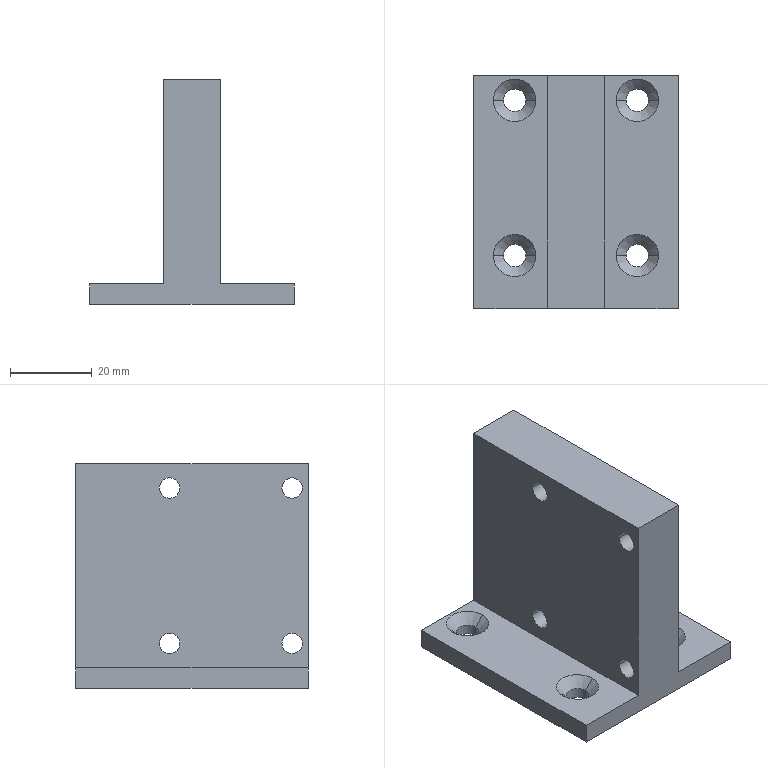Part | 1 solid | 34 faces | box 50 x 57 x 55 mm | volume 52306 mm3 | cylinder 16 | plane 10 | cone 8 | commonest cylinder face diameters 5 x8 5.5 x8
STEP:
#1=CARTESIAN_POINT('',(7.25,41.,2.55));
#2=VERTEX_POINT('',#1);
#3=CARTESIAN_POINT('',(12.75,41.,2.55));
#4=VERTEX_POINT('',#3);
#5=CARTESIAN_POINT('',(10.,41.,2.55));
#6=DIRECTION('',(0.,0.,1.));
#7=DIRECTION('',(1.,0.,0.));
#8=AXIS2_PLACEMENT_3D('',#5,#6,#7);
#9=CIRCLE('',#8,2.75);
#10=EDGE_CURVE('',#2,#4,#9,.T.);
#11=ORIENTED_EDGE('',*,*,#10,.F.);
#12=CARTESIAN_POINT('',(4.8,41.,5.));
#13=VERTEX_POINT('',#12);
#14=CARTESIAN_POINT('',(4.8,41.,5.));
#15=DIRECTION('',(-0.7071,0.,0.7071));
#16=VECTOR('',#15,1000.);
#17=LINE('',#14,#16);
#18=EDGE_CURVE('',#2,#13,#17,.T.);
#19=ORIENTED_EDGE('',*,*,#18,.T.);
#20=CARTESIAN_POINT('',(15.2,41.,5.));
#21=VERTEX_POINT('',#20);
#22=CARTESIAN_POINT('',(10.,41.,5.));
#23=DIRECTION('',(0.,0.,1.));
#24=DIRECTION('',(1.,0.,0.));
#25=AXIS2_PLACEMENT_3D('',#22,#23,#24);
#26=CIRCLE('',#25,5.2);
#27=EDGE_CURVE('',#13,#21,#26,.T.);
#28=ORIENTED_EDGE('',*,*,#27,.T.);
#29=CARTESIAN_POINT('',(15.2,41.,5.));
#30=DIRECTION('',(0.7071,0.,0.7071));
#31=VECTOR('',#30,1000.);
#32=LINE('',#29,#31);
#33=EDGE_CURVE('',#4,#21,#32,.T.);
#34=ORIENTED_EDGE('',*,*,#33,.F.);
#35=EDGE_LOOP('',(#11,#19,#28,#34));
#36=FACE_OUTER_BOUND('',#35,.T.);
#37=CARTESIAN_POINT('',(10.,41.,5.));
#38=DIRECTION('',(0.,0.,1.));
#39=DIRECTION('',(1.,0.,0.));
#40=AXIS2_PLACEMENT_3D('',#37,#38,#39);
#41=CONICAL_SURFACE('',#40,5.2,0.7854);
#42=ADVANCED_FACE('',(#36),#41,.F.);
#43=CARTESIAN_POINT('',(12.75,41.,0.));
#44=VERTEX_POINT('',#43);
#45=CARTESIAN_POINT('',(7.25,41.,0.));
#46=VERTEX_POINT('',#45);
#47=CARTESIAN_POINT('',(10.,41.,0.));
#48=DIRECTION('',(0.,0.,-1.));
#49=DIRECTION('',(-1.,0.,0.));
#50=AXIS2_PLACEMENT_3D('',#47,#48,#49);
#51=CIRCLE('',#50,2.75);
#52=EDGE_CURVE('',#44,#46,#51,.T.);
#53=ORIENTED_EDGE('',*,*,#52,.T.);
#54=CARTESIAN_POINT('',(7.25,41.,5.));
#55=DIRECTION('',(0.,0.,1.));
#56=VECTOR('',#55,1000.);
#57=LINE('',#54,#56);
#58=EDGE_CURVE('',#46,#2,#57,.T.);
#59=ORIENTED_EDGE('',*,*,#58,.T.);
#60=ORIENTED_EDGE('',*,*,#10,.T.);
#61=CARTESIAN_POINT('',(12.75,41.,5.));
#62=DIRECTION('',(0.,0.,1.));
#63=VECTOR('',#62,1000.);
#64=LINE('',#61,#63);
#65=EDGE_CURVE('',#44,#4,#64,.T.);
#66=ORIENTED_EDGE('',*,*,#65,.F.);
#67=EDGE_LOOP('',(#53,#59,#60,#66));
#68=FACE_OUTER_BOUND('',#67,.T.);
#69=CARTESIAN_POINT('',(10.,41.,5.));
#70=DIRECTION('',(0.,0.,1.));
#71=DIRECTION('',(1.,0.,0.));
#72=AXIS2_PLACEMENT_3D('',#69,#70,#71);
#73=CYLINDRICAL_SURFACE('',#72,2.75);
#74=ADVANCED_FACE('',(#68),#73,.F.);
#75=CARTESIAN_POINT('',(7.25,3.,2.55));
#76=VERTEX_POINT('',#75);
#77=CARTESIAN_POINT('',(12.75,3.,2.55));
#78=VERTEX_POINT('',#77);
#79=CARTESIAN_POINT('',(10.,3.,2.55));
#80=DIRECTION('',(0.,0.,1.));
#81=DIRECTION('',(1.,0.,0.));
#82=AXIS2_PLACEMENT_3D('',#79,#80,#81);
#83=CIRCLE('',#82,2.75);
#84=EDGE_CURVE('',#76,#78,#83,.T.);
#85=ORIENTED_EDGE('',*,*,#84,.F.);
#86=CARTESIAN_POINT('',(4.8,3.,5.));
#87=VERTEX_POINT('',#86);
#88=CARTESIAN_POINT('',(4.8,3.,5.));
#89=DIRECTION('',(-0.7071,0.,0.7071));
#90=VECTOR('',#89,1000.);
#91=LINE('',#88,#90);
#92=EDGE_CURVE('',#76,#87,#91,.T.);
#93=ORIENTED_EDGE('',*,*,#92,.T.);
#94=CARTESIAN_POINT('',(15.2,3.,5.));
#95=VERTEX_POINT('',#94);
#96=CARTESIAN_POINT('',(10.,3.,5.));
#97=DIRECTION('',(0.,0.,1.));
#98=DIRECTION('',(1.,0.,0.));
#99=AXIS2_PLACEMENT_3D('',#96,#97,#98);
#100=CIRCLE('',#99,5.2);
#101=EDGE_CURVE('',#87,#95,#100,.T.);
#102=ORIENTED_EDGE('',*,*,#101,.T.);
#103=CARTESIAN_POINT('',(15.2,3.,5.));
#104=DIRECTION('',(0.7071,0.,0.7071));
#105=VECTOR('',#104,1000.);
#106=LINE('',#103,#105);
#107=EDGE_CURVE('',#78,#95,#106,.T.);
#108=ORIENTED_EDGE('',*,*,#107,.F.);
#109=EDGE_LOOP('',(#85,#93,#102,#108));
#110=FACE_OUTER_BOUND('',#109,.T.);
#111=CARTESIAN_POINT('',(10.,3.,5.));
#112=DIRECTION('',(0.,0.,1.));
#113=DIRECTION('',(1.,0.,0.));
#114=AXIS2_PLACEMENT_3D('',#111,#112,#113);
#115=CONICAL_SURFACE('',#114,5.2,0.7854);
#116=ADVANCED_FACE('',(#110),#115,.F.);
#117=CARTESIAN_POINT('',(12.75,3.,0.));
#118=VERTEX_POINT('',#117);
#119=CARTESIAN_POINT('',(7.25,3.,0.));
#120=VERTEX_POINT('',#119);
#121=CARTESIAN_POINT('',(10.,3.,0.));
#122=DIRECTION('',(0.,0.,-1.));
#123=DIRECTION('',(-1.,0.,0.));
#124=AXIS2_PLACEMENT_3D('',#121,#122,#123);
#125=CIRCLE('',#124,2.75);
#126=EDGE_CURVE('',#118,#120,#125,.T.);
#127=ORIENTED_EDGE('',*,*,#126,.T.);
#128=CARTESIAN_POINT('',(7.25,3.,5.));
#129=DIRECTION('',(0.,0.,1.));
#130=VECTOR('',#129,1000.);
#131=LINE('',#128,#130);
#132=EDGE_CURVE('',#120,#76,#131,.T.);
#133=ORIENTED_EDGE('',*,*,#132,.T.);
#134=ORIENTED_EDGE('',*,*,#84,.T.);
#135=CARTESIAN_POINT('',(12.75,3.,5.));
#136=DIRECTION('',(0.,0.,1.));
#137=VECTOR('',#136,1000.);
#138=LINE('',#135,#137);
#139=EDGE_CURVE('',#118,#78,#138,.T.);
#140=ORIENTED_EDGE('',*,*,#139,.F.);
#141=EDGE_LOOP('',(#127,#133,#134,#140));
#142=FACE_OUTER_BOUND('',#141,.T.);
#143=CARTESIAN_POINT('',(10.,3.,5.));
#144=DIRECTION('',(0.,0.,1.));
#145=DIRECTION('',(1.,0.,0.));
#146=AXIS2_PLACEMENT_3D('',#143,#144,#145);
#147=CYLINDRICAL_SURFACE('',#146,2.75);
#148=ADVANCED_FACE('',(#142),#147,.F.);
#149=CARTESIAN_POINT('',(37.25,41.,2.55));
#150=VERTEX_POINT('',#149);
#151=CARTESIAN_POINT('',(42.75,41.,2.55));
#152=VERTEX_POINT('',#151);
#153=CARTESIAN_POINT('',(40.,41.,2.55));
#154=DIRECTION('',(0.,0.,1.));
#155=DIRECTION('',(1.,0.,0.));
#156=AXIS2_PLACEMENT_3D('',#153,#154,#155);
#157=CIRCLE('',#156,2.75);
#158=EDGE_CURVE('',#150,#152,#157,.T.);
#159=ORIENTED_EDGE('',*,*,#158,.F.);
#160=CARTESIAN_POINT('',(34.8,41.,5.));
#161=VERTEX_POINT('',#160);
#162=CARTESIAN_POINT('',(34.8,41.,5.));
#163=DIRECTION('',(-0.7071,0.,0.7071));
#164=VECTOR('',#163,1000.);
#165=LINE('',#162,#164);
#166=EDGE_CURVE('',#150,#161,#165,.T.);
#167=ORIENTED_EDGE('',*,*,#166,.T.);
#168=CARTESIAN_POINT('',(45.2,41.,5.));
#169=VERTEX_POINT('',#168);
#170=CARTESIAN_POINT('',(40.,41.,5.));
#171=DIRECTION('',(0.,0.,1.));
#172=DIRECTION('',(1.,0.,0.));
#173=AXIS2_PLACEMENT_3D('',#170,#171,#172);
#174=CIRCLE('',#173,5.2);
#175=EDGE_CURVE('',#161,#169,#174,.T.);
#176=ORIENTED_EDGE('',*,*,#175,.T.);
#177=CARTESIAN_POINT('',(45.2,41.,5.));
#178=DIRECTION('',(0.7071,0.,0.7071));
#179=VECTOR('',#178,1000.);
#180=LINE('',#177,#179);
#181=EDGE_CURVE('',#152,#169,#180,.T.);
#182=ORIENTED_EDGE('',*,*,#181,.F.);
#183=EDGE_LOOP('',(#159,#167,#176,#182));
#184=FACE_OUTER_BOUND('',#183,.T.);
#185=CARTESIAN_POINT('',(40.,41.,5.));
#186=DIRECTION('',(0.,0.,1.));
#187=DIRECTION('',(1.,0.,0.));
#188=AXIS2_PLACEMENT_3D('',#185,#186,#187);
#189=CONICAL_SURFACE('',#188,5.2,0.7854);
#190=ADVANCED_FACE('',(#184),#189,.F.);
#191=CARTESIAN_POINT('',(42.75,41.,0.));
#192=VERTEX_POINT('',#191);
#193=CARTESIAN_POINT('',(37.25,41.,0.));
#194=VERTEX_POINT('',#193);
#195=CARTESIAN_POINT('',(40.,41.,0.));
#196=DIRECTION('',(0.,0.,-1.));
#197=DIRECTION('',(-1.,0.,0.));
#198=AXIS2_PLACEMENT_3D('',#195,#196,#197);
#199=CIRCLE('',#198,2.75);
#200=EDGE_CURVE('',#192,#194,#199,.T.);
#201=ORIENTED_EDGE('',*,*,#200,.T.);
#202=CARTESIAN_POINT('',(37.25,41.,5.));
#203=DIRECTION('',(0.,0.,1.));
#204=VECTOR('',#203,1000.);
#205=LINE('',#202,#204);
#206=EDGE_CURVE('',#194,#150,#205,.T.);
#207=ORIENTED_EDGE('',*,*,#206,.T.);
#208=ORIENTED_EDGE('',*,*,#158,.T.);
#209=CARTESIAN_POINT('',(42.75,41.,5.));
#210=DIRECTION('',(0.,0.,1.));
#211=VECTOR('',#210,1000.);
#212=LINE('',#209,#211);
#213=EDGE_CURVE('',#192,#152,#212,.T.);
#214=ORIENTED_EDGE('',*,*,#213,.F.);
#215=EDGE_LOOP('',(#201,#207,#208,#214));
#216=FACE_OUTER_BOUND('',#215,.T.);
#217=CARTESIAN_POINT('',(40.,41.,5.));
#218=DIRECTION('',(0.,0.,1.));
#219=DIRECTION('',(1.,0.,0.));
#220=AXIS2_PLACEMENT_3D('',#217,#218,#219);
#221=CYLINDRICAL_SURFACE('',#220,2.75);
#222=ADVANCED_FACE('',(#216),#221,.F.);
#223=CARTESIAN_POINT('',(37.25,3.,2.55));
#224=VERTEX_POINT('',#223);
#225=CARTESIAN_POINT('',(42.75,3.,2.55));
#226=VERTEX_POINT('',#225);
#227=CARTESIAN_POINT('',(40.,3.,2.55));
#228=DIRECTION('',(0.,0.,1.));
#229=DIRECTION('',(1.,0.,0.));
#230=AXIS2_PLACEMENT_3D('',#227,#228,#229);
#231=CIRCLE('',#230,2.75);
#232=EDGE_CURVE('',#224,#226,#231,.T.);
#233=ORIENTED_EDGE('',*,*,#232,.F.);
#234=CARTESIAN_POINT('',(34.8,3.,5.));
#235=VERTEX_POINT('',#234);
#236=CARTESIAN_POINT('',(34.8,3.,5.));
#237=DIRECTION('',(-0.7071,0.,0.7071));
#238=VECTOR('',#237,1000.);
#239=LINE('',#236,#238);
#240=EDGE_CURVE('',#224,#235,#239,.T.);
#241=ORIENTED_EDGE('',*,*,#240,.T.);
#242=CARTESIAN_POINT('',(45.2,3.,5.));
#243=VERTEX_POINT('',#242);
#244=CARTESIAN_POINT('',(40.,3.,5.));
#245=DIRECTION('',(0.,0.,1.));
#246=DIRECTION('',(1.,0.,0.));
#247=AXIS2_PLACEMENT_3D('',#244,#245,#246);
#248=CIRCLE('',#247,5.2);
#249=EDGE_CURVE('',#235,#243,#248,.T.);
#250=ORIENTED_EDGE('',*,*,#249,.T.);
#251=CARTESIAN_POINT('',(45.2,3.,5.));
#252=DIRECTION('',(0.7071,0.,0.7071));
#253=VECTOR('',#252,1000.);
#254=LINE('',#251,#253);
#255=EDGE_CURVE('',#226,#243,#254,.T.);
#256=ORIENTED_EDGE('',*,*,#255,.F.);
#257=EDGE_LOOP('',(#233,#241,#250,#256));
#258=FACE_OUTER_BOUND('',#257,.T.);
#259=CARTESIAN_POINT('',(40.,3.,5.));
#260=DIRECTION('',(0.,0.,1.));
#261=DIRECTION('',(1.,0.,0.));
#262=AXIS2_PLACEMENT_3D('',#259,#260,#261);
#263=CONICAL_SURFACE('',#262,5.2,0.7854);
#264=ADVANCED_FACE('',(#258),#263,.F.);
#265=CARTESIAN_POINT('',(42.75,3.,0.));
#266=VERTEX_POINT('',#265);
#267=CARTESIAN_POINT('',(37.25,3.,0.));
#268=VERTEX_POINT('',#267);
#269=CARTESIAN_POINT('',(40.,3.,0.));
#270=DIRECTION('',(0.,0.,-1.));
#271=DIRECTION('',(-1.,0.,0.));
#272=AXIS2_PLACEMENT_3D('',#269,#270,#271);
#273=CIRCLE('',#272,2.75);
#274=EDGE_CURVE('',#266,#268,#273,.T.);
#275=ORIENTED_EDGE('',*,*,#274,.T.);
#276=CARTESIAN_POINT('',(37.25,3.,5.));
#277=DIRECTION('',(0.,0.,1.));
#278=VECTOR('',#277,1000.);
#279=LINE('',#276,#278);
#280=EDGE_CURVE('',#268,#224,#279,.T.);
#281=ORIENTED_EDGE('',*,*,#280,.T.);
#282=ORIENTED_EDGE('',*,*,#232,.T.);
#283=CARTESIAN_POINT('',(42.75,3.,5.));
#284=DIRECTION('',(0.,0.,1.));
#285=VECTOR('',#284,1000.);
#286=LINE('',#283,#285);
#287=EDGE_CURVE('',#266,#226,#286,.T.);
#288=ORIENTED_EDGE('',*,*,#287,.F.);
#289=EDGE_LOOP('',(#275,#281,#282,#288));
#290=FACE_OUTER_BOUND('',#289,.T.);
#291=CARTESIAN_POINT('',(40.,3.,5.));
#292=DIRECTION('',(0.,0.,1.));
#293=DIRECTION('',(1.,0.,0.));
#294=AXIS2_PLACEMENT_3D('',#291,#292,#293);
#295=CYLINDRICAL_SURFACE('',#294,2.75);
#296=ADVANCED_FACE('',(#290),#295,.F.);
#297=CARTESIAN_POINT('',(32.,-3.5,49.));
#298=VERTEX_POINT('',#297);
#299=CARTESIAN_POINT('',(32.,-8.5,49.));
#300=VERTEX_POINT('',#299);
#301=CARTESIAN_POINT('',(32.,-6.,49.));
#302=DIRECTION('',(-1.,0.,0.));
#303=DIRECTION('',(0.,-1.,0.));
#304=AXIS2_PLACEMENT_3D('',#301,#302,#303);
#305=CIRCLE('',#304,2.5);
#306=EDGE_CURVE('',#298,#300,#305,.T.);
#307=ORIENTED_EDGE('',*,*,#306,.F.);
#308=CARTESIAN_POINT('',(18.,-3.5,49.));
#309=VERTEX_POINT('',#308);
#310=CARTESIAN_POINT('',(50.,-3.5,49.));
#311=DIRECTION('',(-1.,0.,0.));
#312=VECTOR('',#311,1000.);
#313=LINE('',#310,#312);
#314=EDGE_CURVE('',#298,#309,#313,.T.);
#315=ORIENTED_EDGE('',*,*,#314,.T.);
#316=CARTESIAN_POINT('',(18.,-8.5,49.));
#317=VERTEX_POINT('',#316);
#318=CARTESIAN_POINT('',(18.,-6.,49.));
#319=DIRECTION('',(-1.,0.,0.));
#320=DIRECTION('',(0.,-1.,0.));
#321=AXIS2_PLACEMENT_3D('',#318,#319,#320);
#322=CIRCLE('',#321,2.5);
#323=EDGE_CURVE('',#309,#317,#322,.T.);
#324=ORIENTED_EDGE('',*,*,#323,.T.);
#325=CARTESIAN_POINT('',(50.,-8.5,49.));
#326=DIRECTION('',(-1.,0.,0.));
#327=VECTOR('',#326,1000.);
#328=LINE('',#325,#327);
#329=EDGE_CURVE('',#300,#317,#328,.T.);
#330=ORIENTED_EDGE('',*,*,#329,.F.);
#331=EDGE_LOOP('',(#307,#315,#324,#330));
#332=FACE_OUTER_BOUND('',#331,.T.);
#333=CARTESIAN_POINT('',(50.,-6.,49.));
#334=DIRECTION('',(-1.,0.,0.));
#335=DIRECTION('',(0.,-1.,0.));
#336=AXIS2_PLACEMENT_3D('',#333,#334,#335);
#337=CYLINDRICAL_SURFACE('',#336,2.5);
#338=ADVANCED_FACE('',(#332),#337,.F.);
#339=CARTESIAN_POINT('',(32.,-3.5,11.));
#340=VERTEX_POINT('',#339);
#341=CARTESIAN_POINT('',(32.,-8.5,11.));
#342=VERTEX_POINT('',#341);
#343=CARTESIAN_POINT('',(32.,-6.,11.));
#344=DIRECTION('',(-1.,0.,0.));
#345=DIRECTION('',(0.,-1.,0.));
#346=AXIS2_PLACEMENT_3D('',#343,#344,#345);
#347=CIRCLE('',#346,2.5);
#348=EDGE_CURVE('',#340,#342,#347,.T.);
#349=ORIENTED_EDGE('',*,*,#348,.F.);
#350=CARTESIAN_POINT('',(18.,-3.5,11.));
#351=VERTEX_POINT('',#350);
#352=CARTESIAN_POINT('',(50.,-3.5,11.));
#353=DIRECTION('',(-1.,0.,0.));
#354=VECTOR('',#353,1000.);
#355=LINE('',#352,#354);
#356=EDGE_CURVE('',#340,#351,#355,.T.);
#357=ORIENTED_EDGE('',*,*,#356,.T.);
#358=CARTESIAN_POINT('',(18.,-8.5,11.));
#359=VERTEX_POINT('',#358);
#360=CARTESIAN_POINT('',(18.,-6.,11.));
#361=DIRECTION('',(-1.,0.,0.));
#362=DIRECTION('',(0.,-1.,0.));
#363=AXIS2_PLACEMENT_3D('',#360,#361,#362);
#364=CIRCLE('',#363,2.5);
#365=EDGE_CURVE('',#351,#359,#364,.T.);
#366=ORIENTED_EDGE('',*,*,#365,.T.);
#367=CARTESIAN_POINT('',(50.,-8.5,11.));
#368=DIRECTION('',(-1.,0.,0.));
#369=VECTOR('',#368,1000.);
#370=LINE('',#367,#369);
#371=EDGE_CURVE('',#342,#359,#370,.T.);
#372=ORIENTED_EDGE('',*,*,#371,.F.);
#373=EDGE_LOOP('',(#349,#357,#366,#372));
#374=FACE_OUTER_BOUND('',#373,.T.);
#375=CARTESIAN_POINT('',(50.,-6.,11.));
#376=DIRECTION('',(-1.,0.,0.));
#377=DIRECTION('',(0.,-1.,0.));
#378=AXIS2_PLACEMENT_3D('',#375,#376,#377);
#379=CYLINDRICAL_SURFACE('',#378,2.5);
#380=ADVANCED_FACE('',(#374),#379,.F.);
#381=CARTESIAN_POINT('',(32.,26.5,49.));
#382=VERTEX_POINT('',#381);
#383=CARTESIAN_POINT('',(32.,21.5,49.));
#384=VERTEX_POINT('',#383);
#385=CARTESIAN_POINT('',(32.,24.,49.));
#386=DIRECTION('',(-1.,0.,0.));
#387=DIRECTION('',(0.,-1.,0.));
#388=AXIS2_PLACEMENT_3D('',#385,#386,#387);
#389=CIRCLE('',#388,2.5);
#390=EDGE_CURVE('',#382,#384,#389,.T.);
#391=ORIENTED_EDGE('',*,*,#390,.F.);
#392=CARTESIAN_POINT('',(18.,26.5,49.));
#393=VERTEX_POINT('',#392);
#394=CARTESIAN_POINT('',(50.,26.5,49.));
#395=DIRECTION('',(-1.,0.,0.));
#396=VECTOR('',#395,1000.);
#397=LINE('',#394,#396);
#398=EDGE_CURVE('',#382,#393,#397,.T.);
#399=ORIENTED_EDGE('',*,*,#398,.T.);
#400=CARTESIAN_POINT('',(18.,21.5,49.));
#401=VERTEX_POINT('',#400);
#402=CARTESIAN_POINT('',(18.,24.,49.));
#403=DIRECTION('',(-1.,0.,0.));
#404=DIRECTION('',(0.,-1.,0.));
#405=AXIS2_PLACEMENT_3D('',#402,#403,#404);
#406=CIRCLE('',#405,2.5);
#407=EDGE_CURVE('',#393,#401,#406,.T.);
#408=ORIENTED_EDGE('',*,*,#407,.T.);
#409=CARTESIAN_POINT('',(50.,21.5,49.));
#410=DIRECTION('',(-1.,0.,0.));
#411=VECTOR('',#410,1000.);
#412=LINE('',#409,#411);
#413=EDGE_CURVE('',#384,#401,#412,.T.);
#414=ORIENTED_EDGE('',*,*,#413,.F.);
#415=EDGE_LOOP('',(#391,#399,#408,#414));
#416=FACE_OUTER_BOUND('',#415,.T.);
#417=CARTESIAN_POINT('',(50.,24.,49.));
#418=DIRECTION('',(-1.,0.,0.));
#419=DIRECTION('',(0.,-1.,0.));
#420=AXIS2_PLACEMENT_3D('',#417,#418,#419);
#421=CYLINDRICAL_SURFACE('',#420,2.5);
#422=ADVANCED_FACE('',(#416),#421,.F.);
#423=CARTESIAN_POINT('',(32.,26.5,11.));
#424=VERTEX_POINT('',#423);
#425=CARTESIAN_POINT('',(32.,21.5,11.));
#426=VERTEX_POINT('',#425);
#427=CARTESIAN_POINT('',(32.,24.,11.));
#428=DIRECTION('',(-1.,0.,0.));
#429=DIRECTION('',(0.,-1.,0.));
#430=AXIS2_PLACEMENT_3D('',#427,#428,#429);
#431=CIRCLE('',#430,2.5);
#432=EDGE_CURVE('',#424,#426,#431,.T.);
#433=ORIENTED_EDGE('',*,*,#432,.F.);
#434=CARTESIAN_POINT('',(18.,26.5,11.));
#435=VERTEX_POINT('',#434);
#436=CARTESIAN_POINT('',(50.,26.5,11.));
#437=DIRECTION('',(-1.,0.,0.));
#438=VECTOR('',#437,1000.);
#439=LINE('',#436,#438);
#440=EDGE_CURVE('',#424,#435,#439,.T.);
#441=ORIENTED_EDGE('',*,*,#440,.T.);
#442=CARTESIAN_POINT('',(18.,21.5,11.));
#443=VERTEX_POINT('',#442);
#444=CARTESIAN_POINT('',(18.,24.,11.));
#445=DIRECTION('',(-1.,0.,0.));
#446=DIRECTION('',(0.,-1.,0.));
#447=AXIS2_PLACEMENT_3D('',#444,#445,#446);
#448=CIRCLE('',#447,2.5);
#449=EDGE_CURVE('',#435,#443,#448,.T.);
#450=ORIENTED_EDGE('',*,*,#449,.T.);
#451=CARTESIAN_POINT('',(50.,21.5,11.));
#452=DIRECTION('',(-1.,0.,0.));
#453=VECTOR('',#452,1000.);
#454=LINE('',#451,#453);
#455=EDGE_CURVE('',#426,#443,#454,.T.);
#456=ORIENTED_EDGE('',*,*,#455,.F.);
#457=EDGE_LOOP('',(#433,#441,#450,#456));
#458=FACE_OUTER_BOUND('',#457,.T.);
#459=CARTESIAN_POINT('',(50.,24.,11.));
#460=DIRECTION('',(-1.,0.,0.));
#461=DIRECTION('',(0.,-1.,0.));
#462=AXIS2_PLACEMENT_3D('',#459,#460,#461);
#463=CYLINDRICAL_SURFACE('',#462,2.5);
#464=ADVANCED_FACE('',(#458),#463,.F.);
#465=CARTESIAN_POINT('',(10.,41.,5.));
#466=DIRECTION('',(0.,0.,1.));
#467=DIRECTION('',(1.,0.,0.));
#468=AXIS2_PLACEMENT_3D('',#465,#466,#467);
#469=CIRCLE('',#468,5.2);
#470=EDGE_CURVE('',#21,#13,#469,.T.);
#471=ORIENTED_EDGE('',*,*,#470,.F.);
#472=ORIENTED_EDGE('',*,*,#27,.F.);
#473=EDGE_LOOP('',(#471,#472));
#474=FACE_BOUND('',#473,.T.);
#475=CARTESIAN_POINT('',(10.,3.,5.));
#476=DIRECTION('',(0.,0.,1.));
#477=DIRECTION('',(1.,0.,0.));
#478=AXIS2_PLACEMENT_3D('',#475,#476,#477);
#479=CIRCLE('',#478,5.2);
#480=EDGE_CURVE('',#95,#87,#479,.T.);
#481=ORIENTED_EDGE('',*,*,#480,.F.);
#482=ORIENTED_EDGE('',*,*,#101,.F.);
#483=EDGE_LOOP('',(#481,#482));
#484=FACE_BOUND('',#483,.T.);
#485=CARTESIAN_POINT('',(18.,47.,5.));
#486=VERTEX_POINT('',#485);
#487=CARTESIAN_POINT('',(18.,-10.,5.));
#488=VERTEX_POINT('',#487);
#489=CARTESIAN_POINT('',(18.,47.,5.));
#490=DIRECTION('',(0.,-1.,0.));
#491=VECTOR('',#490,1000.);
#492=LINE('',#489,#491);
#493=EDGE_CURVE('',#486,#488,#492,.T.);
#494=ORIENTED_EDGE('',*,*,#493,.F.);
#495=CARTESIAN_POINT('',(0.,47.,5.));
#496=VERTEX_POINT('',#495);
#497=CARTESIAN_POINT('',(0.,47.,5.));
#498=DIRECTION('',(-1.,0.,0.));
#499=VECTOR('',#498,1000.);
#500=LINE('',#497,#499);
#501=EDGE_CURVE('',#486,#496,#500,.T.);
#502=ORIENTED_EDGE('',*,*,#501,.T.);
#503=CARTESIAN_POINT('',(0.,-10.,5.));
#504=VERTEX_POINT('',#503);
#505=CARTESIAN_POINT('',(0.,0.,5.));
#506=DIRECTION('',(0.,-1.,0.));
#507=VECTOR('',#506,1000.);
#508=LINE('',#505,#507);
#509=EDGE_CURVE('',#496,#504,#508,.T.);
#510=ORIENTED_EDGE('',*,*,#509,.T.);
#511=CARTESIAN_POINT('',(18.,-10.,5.));
#512=DIRECTION('',(-1.,0.,0.));
#513=VECTOR('',#512,1000.);
#514=LINE('',#511,#513);
#515=EDGE_CURVE('',#488,#504,#514,.T.);
#516=ORIENTED_EDGE('',*,*,#515,.F.);
#517=EDGE_LOOP('',(#494,#502,#510,#516));
#518=FACE_OUTER_BOUND('',#517,.T.);
#519=CARTESIAN_POINT('',(0.,0.,5.));
#520=DIRECTION('',(0.,0.,-1.));
#521=DIRECTION('',(-1.,0.,0.));
#522=AXIS2_PLACEMENT_3D('',#519,#520,#521);
#523=PLANE('',#522);
#524=ADVANCED_FACE('',(#474,#484,#518),#523,.F.);
#525=CARTESIAN_POINT('',(40.,41.,5.));
#526=DIRECTION('',(0.,0.,1.));
#527=DIRECTION('',(1.,0.,0.));
#528=AXIS2_PLACEMENT_3D('',#525,#526,#527);
#529=CIRCLE('',#528,5.2);
#530=EDGE_CURVE('',#169,#161,#529,.T.);
#531=ORIENTED_EDGE('',*,*,#530,.F.);
#532=ORIENTED_EDGE('',*,*,#175,.F.);
#533=EDGE_LOOP('',(#531,#532));
#534=FACE_BOUND('',#533,.T.);
#535=CARTESIAN_POINT('',(40.,3.,5.));
#536=DIRECTION('',(0.,0.,1.));
#537=DIRECTION('',(1.,0.,0.));
#538=AXIS2_PLACEMENT_3D('',#535,#536,#537);
#539=CIRCLE('',#538,5.2);
#540=EDGE_CURVE('',#243,#235,#539,.T.);
#541=ORIENTED_EDGE('',*,*,#540,.F.);
#542=ORIENTED_EDGE('',*,*,#249,.F.);
#543=EDGE_LOOP('',(#541,#542));
#544=FACE_BOUND('',#543,.T.);
#545=CARTESIAN_POINT('',(32.,-10.,5.));
#546=VERTEX_POINT('',#545);
#547=CARTESIAN_POINT('',(32.,47.,5.));
#548=VERTEX_POINT('',#547);
#549=CARTESIAN_POINT('',(32.,47.,5.));
#550=DIRECTION('',(0.,1.,0.));
#551=VECTOR('',#550,1000.);
#552=LINE('',#549,#551);
#553=EDGE_CURVE('',#546,#548,#552,.T.);
#554=ORIENTED_EDGE('',*,*,#553,.F.);
#555=CARTESIAN_POINT('',(50.,-10.,5.));
#556=VERTEX_POINT('',#555);
#557=CARTESIAN_POINT('',(50.,-10.,5.));
#558=DIRECTION('',(-1.,0.,0.));
#559=VECTOR('',#558,1000.);
#560=LINE('',#557,#559);
#561=EDGE_CURVE('',#556,#546,#560,.T.);
#562=ORIENTED_EDGE('',*,*,#561,.F.);
#563=CARTESIAN_POINT('',(50.,47.,5.));
#564=VERTEX_POINT('',#563);
#565=CARTESIAN_POINT('',(50.,0.,5.));
#566=DIRECTION('',(0.,1.,0.));
#567=VECTOR('',#566,1000.);
#568=LINE('',#565,#567);
#569=EDGE_CURVE('',#556,#564,#568,.T.);
#570=ORIENTED_EDGE('',*,*,#569,.T.);
#571=CARTESIAN_POINT('',(0.,47.,5.));
#572=DIRECTION('',(-1.,0.,0.));
#573=VECTOR('',#572,1000.);
#574=LINE('',#571,#573);
#575=EDGE_CURVE('',#564,#548,#574,.T.);
#576=ORIENTED_EDGE('',*,*,#575,.T.);
#577=EDGE_LOOP('',(#554,#562,#570,#576));
#578=FACE_OUTER_BOUND('',#577,.T.);
#579=CARTESIAN_POINT('',(0.,0.,5.));
#580=DIRECTION('',(0.,0.,-1.));
#581=DIRECTION('',(-1.,0.,0.));
#582=AXIS2_PLACEMENT_3D('',#579,#580,#581);
#583=PLANE('',#582);
#584=ADVANCED_FACE('',(#534,#544,#578),#583,.F.);
#585=CARTESIAN_POINT('',(0.,47.,0.));
#586=VERTEX_POINT('',#585);
#587=CARTESIAN_POINT('',(0.,-10.,0.));
#588=VERTEX_POINT('',#587);
#589=CARTESIAN_POINT('',(0.,0.,0.));
#590=DIRECTION('',(0.,-1.,0.));
#591=VECTOR('',#590,1000.);
#592=LINE('',#589,#591);
#593=EDGE_CURVE('',#586,#588,#592,.T.);
#594=ORIENTED_EDGE('',*,*,#593,.T.);
#595=CARTESIAN_POINT('',(0.,-10.,5.));
#596=DIRECTION('',(0.,0.,-1.));
#597=VECTOR('',#596,1000.);
#598=LINE('',#595,#597);
#599=EDGE_CURVE('',#504,#588,#598,.T.);
#600=ORIENTED_EDGE('',*,*,#599,.F.);
#601=ORIENTED_EDGE('',*,*,#509,.F.);
#602=CARTESIAN_POINT('',(0.,47.,5.));
#603=DIRECTION('',(0.,0.,-1.));
#604=VECTOR('',#603,1000.);
#605=LINE('',#602,#604);
#606=EDGE_CURVE('',#496,#586,#605,.T.);
#607=ORIENTED_EDGE('',*,*,#606,.T.);
#608=EDGE_LOOP('',(#594,#600,#601,#607));
#609=FACE_OUTER_BOUND('',#608,.T.);
#610=CARTESIAN_POINT('',(0.,0.,5.));
#611=DIRECTION('',(1.,0.,0.));
#612=DIRECTION('',(0.,0.,-1.));
#613=AXIS2_PLACEMENT_3D('',#610,#611,#612);
#614=PLANE('',#613);
#615=ADVANCED_FACE('',(#609),#614,.F.);
#616=CARTESIAN_POINT('',(50.,-10.,0.));
#617=VERTEX_POINT('',#616);
#618=CARTESIAN_POINT('',(50.,47.,0.));
#619=VERTEX_POINT('',#618);
#620=CARTESIAN_POINT('',(50.,0.,0.));
#621=DIRECTION('',(0.,1.,0.));
#622=VECTOR('',#621,1000.);
#623=LINE('',#620,#622);
#624=EDGE_CURVE('',#617,#619,#623,.T.);
#625=ORIENTED_EDGE('',*,*,#624,.T.);
#626=CARTESIAN_POINT('',(50.,47.,5.));
#627=DIRECTION('',(0.,0.,-1.));
#628=VECTOR('',#627,1000.);
#629=LINE('',#626,#628);
#630=EDGE_CURVE('',#564,#619,#629,.T.);
#631=ORIENTED_EDGE('',*,*,#630,.F.);
#632=ORIENTED_EDGE('',*,*,#569,.F.);
#633=CARTESIAN_POINT('',(50.,-10.,0.));
#634=DIRECTION('',(0.,0.,1.));
#635=VECTOR('',#634,1000.);
#636=LINE('',#633,#635);
#637=EDGE_CURVE('',#617,#556,#636,.T.);
#638=ORIENTED_EDGE('',*,*,#637,.F.);
#639=EDGE_LOOP('',(#625,#631,#632,#638));
#640=FACE_OUTER_BOUND('',#639,.T.);
#641=CARTESIAN_POINT('',(50.,0.,5.));
#642=DIRECTION('',(-1.,0.,0.));
#643=DIRECTION('',(0.,0.,1.));
#644=AXIS2_PLACEMENT_3D('',#641,#642,#643);
#645=PLANE('',#644);
#646=ADVANCED_FACE('',(#640),#645,.F.);
#647=CARTESIAN_POINT('',(0.,47.,0.));
#648=DIRECTION('',(-1.,0.,0.));
#649=VECTOR('',#648,1000.);
#650=LINE('',#647,#649);
#651=EDGE_CURVE('',#619,#586,#650,.T.);
#652=ORIENTED_EDGE('',*,*,#651,.T.);
#653=ORIENTED_EDGE('',*,*,#606,.F.);
#654=ORIENTED_EDGE('',*,*,#501,.F.);
#655=CARTESIAN_POINT('',(18.,47.,55.));
#656=VERTEX_POINT('',#655);
#657=CARTESIAN_POINT('',(18.,47.,55.));
#658=DIRECTION('',(0.,0.,-1.));
#659=VECTOR('',#658,1000.);
#660=LINE('',#657,#659);
#661=EDGE_CURVE('',#656,#486,#660,.T.);
#662=ORIENTED_EDGE('',*,*,#661,.F.);
#663=CARTESIAN_POINT('',(32.,47.,55.));
#664=VERTEX_POINT('',#663);
#665=CARTESIAN_POINT('',(18.,47.,55.));
#666=DIRECTION('',(-1.,0.,0.));
#667=VECTOR('',#666,1000.);
#668=LINE('',#665,#667);
#669=EDGE_CURVE('',#664,#656,#668,.T.);
#670=ORIENTED_EDGE('',*,*,#669,.F.);
#671=CARTESIAN_POINT('',(32.,47.,55.));
#672=DIRECTION('',(0.,0.,-1.));
#673=VECTOR('',#672,1000.);
#674=LINE('',#671,#673);
#675=EDGE_CURVE('',#664,#548,#674,.T.);
#676=ORIENTED_EDGE('',*,*,#675,.T.);
#677=ORIENTED_EDGE('',*,*,#575,.F.);
#678=ORIENTED_EDGE('',*,*,#630,.T.);
#679=EDGE_LOOP('',(#652,#653,#654,#662,#670,#676,#677,#678));
#680=FACE_OUTER_BOUND('',#679,.T.);
#681=CARTESIAN_POINT('',(0.,47.,5.));
#682=DIRECTION('',(0.,-1.,0.));
#683=DIRECTION('',(0.,0.,-1.));
#684=AXIS2_PLACEMENT_3D('',#681,#682,#683);
#685=PLANE('',#684);
#686=ADVANCED_FACE('',(#680),#685,.F.);
#687=ORIENTED_EDGE('',*,*,#52,.F.);
#688=CARTESIAN_POINT('',(10.,41.,0.));
#689=DIRECTION('',(0.,0.,-1.));
#690=DIRECTION('',(-1.,0.,0.));
#691=AXIS2_PLACEMENT_3D('',#688,#689,#690);
#692=CIRCLE('',#691,2.75);
#693=EDGE_CURVE('',#46,#44,#692,.T.);
#694=ORIENTED_EDGE('',*,*,#693,.F.);
#695=EDGE_LOOP('',(#687,#694));
#696=FACE_BOUND('',#695,.T.);
#697=ORIENTED_EDGE('',*,*,#126,.F.);
#698=CARTESIAN_POINT('',(10.,3.,0.));
#699=DIRECTION('',(0.,0.,-1.));
#700=DIRECTION('',(-1.,0.,0.));
#701=AXIS2_PLACEMENT_3D('',#698,#699,#700);
#702=CIRCLE('',#701,2.75);
#703=EDGE_CURVE('',#120,#118,#702,.T.);
#704=ORIENTED_EDGE('',*,*,#703,.F.);
#705=EDGE_LOOP('',(#697,#704));
#706=FACE_BOUND('',#705,.T.);
#707=ORIENTED_EDGE('',*,*,#200,.F.);
#708=CARTESIAN_POINT('',(40.,41.,0.));
#709=DIRECTION('',(0.,0.,-1.));
#710=DIRECTION('',(-1.,0.,0.));
#711=AXIS2_PLACEMENT_3D('',#708,#709,#710);
#712=CIRCLE('',#711,2.75);
#713=EDGE_CURVE('',#194,#192,#712,.T.);
#714=ORIENTED_EDGE('',*,*,#713,.F.);
#715=EDGE_LOOP('',(#707,#714));
#716=FACE_BOUND('',#715,.T.);
#717=ORIENTED_EDGE('',*,*,#274,.F.);
#718=CARTESIAN_POINT('',(40.,3.,0.));
#719=DIRECTION('',(0.,0.,-1.));
#720=DIRECTION('',(-1.,0.,0.));
#721=AXIS2_PLACEMENT_3D('',#718,#719,#720);
#722=CIRCLE('',#721,2.75);
#723=EDGE_CURVE('',#268,#266,#722,.T.);
#724=ORIENTED_EDGE('',*,*,#723,.F.);
#725=EDGE_LOOP('',(#717,#724));
#726=FACE_BOUND('',#725,.T.);
#727=ORIENTED_EDGE('',*,*,#593,.F.);
#728=ORIENTED_EDGE('',*,*,#651,.F.);
#729=ORIENTED_EDGE('',*,*,#624,.F.);
#730=CARTESIAN_POINT('',(0.,-10.,0.));
#731=DIRECTION('',(1.,0.,0.));
#732=VECTOR('',#731,1000.);
#733=LINE('',#730,#732);
#734=EDGE_CURVE('',#588,#617,#733,.T.);
#735=ORIENTED_EDGE('',*,*,#734,.F.);
#736=EDGE_LOOP('',(#727,#728,#729,#735));
#737=FACE_OUTER_BOUND('',#736,.T.);
#738=CARTESIAN_POINT('',(0.,0.,0.));
#739=DIRECTION('',(0.,0.,-1.));
#740=DIRECTION('',(-1.,0.,0.));
#741=AXIS2_PLACEMENT_3D('',#738,#739,#740);
#742=PLANE('',#741);
#743=ADVANCED_FACE('',(#696,#706,#716,#726,#737),#742,.T.);
#744=CARTESIAN_POINT('',(18.,-6.,49.));
#745=DIRECTION('',(-1.,0.,0.));
#746=DIRECTION('',(0.,-1.,0.));
#747=AXIS2_PLACEMENT_3D('',#744,#745,#746);
#748=CIRCLE('',#747,2.5);
#749=EDGE_CURVE('',#317,#309,#748,.T.);
#750=ORIENTED_EDGE('',*,*,#749,.F.);
#751=ORIENTED_EDGE('',*,*,#323,.F.);
#752=EDGE_LOOP('',(#750,#751));
#753=FACE_BOUND('',#752,.T.);
#754=CARTESIAN_POINT('',(18.,-6.,11.));
#755=DIRECTION('',(-1.,0.,0.));
#756=DIRECTION('',(0.,-1.,0.));
#757=AXIS2_PLACEMENT_3D('',#754,#755,#756);
#758=CIRCLE('',#757,2.5);
#759=EDGE_CURVE('',#359,#351,#758,.T.);
#760=ORIENTED_EDGE('',*,*,#759,.F.);
#761=ORIENTED_EDGE('',*,*,#365,.F.);
#762=EDGE_LOOP('',(#760,#761));
#763=FACE_BOUND('',#762,.T.);
#764=CARTESIAN_POINT('',(18.,24.,49.));
#765=DIRECTION('',(-1.,0.,0.));
#766=DIRECTION('',(0.,-1.,0.));
#767=AXIS2_PLACEMENT_3D('',#764,#765,#766);
#768=CIRCLE('',#767,2.5);
#769=EDGE_CURVE('',#401,#393,#768,.T.);
#770=ORIENTED_EDGE('',*,*,#769,.F.);
#771=ORIENTED_EDGE('',*,*,#407,.F.);
#772=EDGE_LOOP('',(#770,#771));
#773=FACE_BOUND('',#772,.T.);
#774=CARTESIAN_POINT('',(18.,24.,11.));
#775=DIRECTION('',(-1.,0.,0.));
#776=DIRECTION('',(0.,-1.,0.));
#777=AXIS2_PLACEMENT_3D('',#774,#775,#776);
#778=CIRCLE('',#777,2.5);
#779=EDGE_CURVE('',#443,#435,#778,.T.);
#780=ORIENTED_EDGE('',*,*,#779,.F.);
#781=ORIENTED_EDGE('',*,*,#449,.F.);
#782=EDGE_LOOP('',(#780,#781));
#783=FACE_BOUND('',#782,.T.);
#784=ORIENTED_EDGE('',*,*,#493,.T.);
#785=CARTESIAN_POINT('',(18.,-10.,55.));
#786=VERTEX_POINT('',#785);
#787=CARTESIAN_POINT('',(18.,-10.,55.));
#788=DIRECTION('',(0.,0.,-1.));
#789=VECTOR('',#788,1000.);
#790=LINE('',#787,#789);
#791=EDGE_CURVE('',#786,#488,#790,.T.);
#792=ORIENTED_EDGE('',*,*,#791,.F.);
#793=CARTESIAN_POINT('',(18.,47.,55.));
#794=DIRECTION('',(0.,-1.,0.));
#795=VECTOR('',#794,1000.);
#796=LINE('',#793,#795);
#797=EDGE_CURVE('',#656,#786,#796,.T.);
#798=ORIENTED_EDGE('',*,*,#797,.F.);
#799=ORIENTED_EDGE('',*,*,#661,.T.);
#800=EDGE_LOOP('',(#784,#792,#798,#799));
#801=FACE_OUTER_BOUND('',#800,.T.);
#802=CARTESIAN_POINT('',(18.,47.,55.));
#803=DIRECTION('',(1.,0.,0.));
#804=DIRECTION('',(0.,1.,0.));
#805=AXIS2_PLACEMENT_3D('',#802,#803,#804);
#806=PLANE('',#805);
#807=ADVANCED_FACE('',(#753,#763,#773,#783,#801),#806,.F.);
#808=CARTESIAN_POINT('',(32.,-6.,49.));
#809=DIRECTION('',(-1.,0.,0.));
#810=DIRECTION('',(0.,-1.,0.));
#811=AXIS2_PLACEMENT_3D('',#808,#809,#810);
#812=CIRCLE('',#811,2.5);
#813=EDGE_CURVE('',#300,#298,#812,.T.);
#814=ORIENTED_EDGE('',*,*,#813,.T.);
#815=ORIENTED_EDGE('',*,*,#306,.T.);
#816=EDGE_LOOP('',(#814,#815));
#817=FACE_BOUND('',#816,.T.);
#818=CARTESIAN_POINT('',(32.,-6.,11.));
#819=DIRECTION('',(-1.,0.,0.));
#820=DIRECTION('',(0.,-1.,0.));
#821=AXIS2_PLACEMENT_3D('',#818,#819,#820);
#822=CIRCLE('',#821,2.5);
#823=EDGE_CURVE('',#342,#340,#822,.T.);
#824=ORIENTED_EDGE('',*,*,#823,.T.);
#825=ORIENTED_EDGE('',*,*,#348,.T.);
#826=EDGE_LOOP('',(#824,#825));
#827=FACE_BOUND('',#826,.T.);
#828=CARTESIAN_POINT('',(32.,24.,49.));
#829=DIRECTION('',(-1.,0.,0.));
#830=DIRECTION('',(0.,-1.,0.));
#831=AXIS2_PLACEMENT_3D('',#828,#829,#830);
#832=CIRCLE('',#831,2.5);
#833=EDGE_CURVE('',#384,#382,#832,.T.);
#834=ORIENTED_EDGE('',*,*,#833,.T.);
#835=ORIENTED_EDGE('',*,*,#390,.T.);
#836=EDGE_LOOP('',(#834,#835));
#837=FACE_BOUND('',#836,.T.);
#838=CARTESIAN_POINT('',(32.,24.,11.));
#839=DIRECTION('',(-1.,0.,0.));
#840=DIRECTION('',(0.,-1.,0.));
#841=AXIS2_PLACEMENT_3D('',#838,#839,#840);
#842=CIRCLE('',#841,2.5);
#843=EDGE_CURVE('',#426,#424,#842,.T.);
#844=ORIENTED_EDGE('',*,*,#843,.T.);
#845=ORIENTED_EDGE('',*,*,#432,.T.);
#846=EDGE_LOOP('',(#844,#845));
#847=FACE_BOUND('',#846,.T.);
#848=ORIENTED_EDGE('',*,*,#553,.T.);
#849=ORIENTED_EDGE('',*,*,#675,.F.);
#850=CARTESIAN_POINT('',(32.,-10.,55.));
#851=VERTEX_POINT('',#850);
#852=CARTESIAN_POINT('',(32.,47.,55.));
#853=DIRECTION('',(0.,1.,0.));
#854=VECTOR('',#853,1000.);
#855=LINE('',#852,#854);
#856=EDGE_CURVE('',#851,#664,#855,.T.);
#857=ORIENTED_EDGE('',*,*,#856,.F.);
#858=CARTESIAN_POINT('',(32.,-10.,5.));
#859=DIRECTION('',(0.,0.,1.));
#860=VECTOR('',#859,1000.);
#861=LINE('',#858,#860);
#862=EDGE_CURVE('',#546,#851,#861,.T.);
#863=ORIENTED_EDGE('',*,*,#862,.F.);
#864=EDGE_LOOP('',(#848,#849,#857,#863));
#865=FACE_OUTER_BOUND('',#864,.T.);
#866=CARTESIAN_POINT('',(32.,47.,55.));
#867=DIRECTION('',(-1.,0.,0.));
#868=DIRECTION('',(0.,-1.,0.));
#869=AXIS2_PLACEMENT_3D('',#866,#867,#868);
#870=PLANE('',#869);
#871=ADVANCED_FACE('',(#817,#827,#837,#847,#865),#870,.F.);
#872=ORIENTED_EDGE('',*,*,#797,.T.);
#873=CARTESIAN_POINT('',(32.,-10.,55.));
#874=DIRECTION('',(-1.,0.,0.));
#875=VECTOR('',#874,1000.);
#876=LINE('',#873,#875);
#877=EDGE_CURVE('',#851,#786,#876,.T.);
#878=ORIENTED_EDGE('',*,*,#877,.F.);
#879=ORIENTED_EDGE('',*,*,#856,.T.);
#880=ORIENTED_EDGE('',*,*,#669,.T.);
#881=EDGE_LOOP('',(#872,#878,#879,#880));
#882=FACE_OUTER_BOUND('',#881,.T.);
#883=CARTESIAN_POINT('',(0.,0.,55.));
#884=DIRECTION('',(0.,0.,1.));
#885=DIRECTION('',(1.,0.,0.));
#886=AXIS2_PLACEMENT_3D('',#883,#884,#885);
#887=PLANE('',#886);
#888=ADVANCED_FACE('',(#882),#887,.T.);
#889=ORIENTED_EDGE('',*,*,#599,.T.);
#890=ORIENTED_EDGE('',*,*,#734,.T.);
#891=ORIENTED_EDGE('',*,*,#637,.T.);
#892=ORIENTED_EDGE('',*,*,#561,.T.);
#893=ORIENTED_EDGE('',*,*,#862,.T.);
#894=ORIENTED_EDGE('',*,*,#877,.T.);
#895=ORIENTED_EDGE('',*,*,#791,.T.);
#896=ORIENTED_EDGE('',*,*,#515,.T.);
#897=EDGE_LOOP('',(#889,#890,#891,#892,#893,#894,#895,#896));
#898=FACE_OUTER_BOUND('',#897,.T.);
#899=CARTESIAN_POINT('',(0.,-10.,0.));
#900=DIRECTION('',(0.,-1.,0.));
#901=DIRECTION('',(0.,0.,-1.));
#902=AXIS2_PLACEMENT_3D('',#899,#900,#901);
#903=PLANE('',#902);
#904=ADVANCED_FACE('',(#898),#903,.T.);
#905=ORIENTED_EDGE('',*,*,#440,.F.);
#906=ORIENTED_EDGE('',*,*,#843,.F.);
#907=ORIENTED_EDGE('',*,*,#455,.T.);
#908=ORIENTED_EDGE('',*,*,#779,.T.);
#909=EDGE_LOOP('',(#905,#906,#907,#908));
#910=FACE_OUTER_BOUND('',#909,.T.);
#911=CARTESIAN_POINT('',(50.,24.,11.));
#912=DIRECTION('',(-1.,0.,0.));
#913=DIRECTION('',(0.,-1.,0.));
#914=AXIS2_PLACEMENT_3D('',#911,#912,#913);
#915=CYLINDRICAL_SURFACE('',#914,2.5);
#916=ADVANCED_FACE('',(#910),#915,.F.);
#917=ORIENTED_EDGE('',*,*,#398,.F.);
#918=ORIENTED_EDGE('',*,*,#833,.F.);
#919=ORIENTED_EDGE('',*,*,#413,.T.);
#920=ORIENTED_EDGE('',*,*,#769,.T.);
#921=EDGE_LOOP('',(#917,#918,#919,#920));
#922=FACE_OUTER_BOUND('',#921,.T.);
#923=CARTESIAN_POINT('',(50.,24.,49.));
#924=DIRECTION('',(-1.,0.,0.));
#925=DIRECTION('',(0.,-1.,0.));
#926=AXIS2_PLACEMENT_3D('',#923,#924,#925);
#927=CYLINDRICAL_SURFACE('',#926,2.5);
#928=ADVANCED_FACE('',(#922),#927,.F.);
#929=ORIENTED_EDGE('',*,*,#356,.F.);
#930=ORIENTED_EDGE('',*,*,#823,.F.);
#931=ORIENTED_EDGE('',*,*,#371,.T.);
#932=ORIENTED_EDGE('',*,*,#759,.T.);
#933=EDGE_LOOP('',(#929,#930,#931,#932));
#934=FACE_OUTER_BOUND('',#933,.T.);
#935=CARTESIAN_POINT('',(50.,-6.,11.));
#936=DIRECTION('',(-1.,0.,0.));
#937=DIRECTION('',(0.,-1.,0.));
#938=AXIS2_PLACEMENT_3D('',#935,#936,#937);
#939=CYLINDRICAL_SURFACE('',#938,2.5);
#940=ADVANCED_FACE('',(#934),#939,.F.);
#941=ORIENTED_EDGE('',*,*,#314,.F.);
#942=ORIENTED_EDGE('',*,*,#813,.F.);
#943=ORIENTED_EDGE('',*,*,#329,.T.);
#944=ORIENTED_EDGE('',*,*,#749,.T.);
#945=EDGE_LOOP('',(#941,#942,#943,#944));
#946=FACE_OUTER_BOUND('',#945,.T.);
#947=CARTESIAN_POINT('',(50.,-6.,49.));
#948=DIRECTION('',(-1.,0.,0.));
#949=DIRECTION('',(0.,-1.,0.));
#950=AXIS2_PLACEMENT_3D('',#947,#948,#949);
#951=CYLINDRICAL_SURFACE('',#950,2.5);
#952=ADVANCED_FACE('',(#946),#951,.F.);
#953=ORIENTED_EDGE('',*,*,#280,.F.);
#954=ORIENTED_EDGE('',*,*,#723,.T.);
#955=ORIENTED_EDGE('',*,*,#287,.T.);
#956=CARTESIAN_POINT('',(40.,3.,2.55));
#957=DIRECTION('',(0.,0.,1.));
#958=DIRECTION('',(1.,0.,0.));
#959=AXIS2_PLACEMENT_3D('',#956,#957,#958);
#960=CIRCLE('',#959,2.75);
#961=EDGE_CURVE('',#226,#224,#960,.T.);
#962=ORIENTED_EDGE('',*,*,#961,.T.);
#963=EDGE_LOOP('',(#953,#954,#955,#962));
#964=FACE_OUTER_BOUND('',#963,.T.);
#965=CARTESIAN_POINT('',(40.,3.,5.));
#966=DIRECTION('',(0.,0.,1.));
#967=DIRECTION('',(1.,0.,0.));
#968=AXIS2_PLACEMENT_3D('',#965,#966,#967);
#969=CYLINDRICAL_SURFACE('',#968,2.75);
#970=ADVANCED_FACE('',(#964),#969,.F.);
#971=ORIENTED_EDGE('',*,*,#240,.F.);
#972=ORIENTED_EDGE('',*,*,#961,.F.);
#973=ORIENTED_EDGE('',*,*,#255,.T.);
#974=ORIENTED_EDGE('',*,*,#540,.T.);
#975=EDGE_LOOP('',(#971,#972,#973,#974));
#976=FACE_OUTER_BOUND('',#975,.T.);
#977=CARTESIAN_POINT('',(40.,3.,5.));
#978=DIRECTION('',(0.,0.,1.));
#979=DIRECTION('',(1.,0.,0.));
#980=AXIS2_PLACEMENT_3D('',#977,#978,#979);
#981=CONICAL_SURFACE('',#980,5.2,0.7854);
#982=ADVANCED_FACE('',(#976),#981,.F.);
#983=ORIENTED_EDGE('',*,*,#206,.F.);
#984=ORIENTED_EDGE('',*,*,#713,.T.);
#985=ORIENTED_EDGE('',*,*,#213,.T.);
#986=CARTESIAN_POINT('',(40.,41.,2.55));
#987=DIRECTION('',(0.,0.,1.));
#988=DIRECTION('',(1.,0.,0.));
#989=AXIS2_PLACEMENT_3D('',#986,#987,#988);
#990=CIRCLE('',#989,2.75);
#991=EDGE_CURVE('',#152,#150,#990,.T.);
#992=ORIENTED_EDGE('',*,*,#991,.T.);
#993=EDGE_LOOP('',(#983,#984,#985,#992));
#994=FACE_OUTER_BOUND('',#993,.T.);
#995=CARTESIAN_POINT('',(40.,41.,5.));
#996=DIRECTION('',(0.,0.,1.));
#997=DIRECTION('',(1.,0.,0.));
#998=AXIS2_PLACEMENT_3D('',#995,#996,#997);
#999=CYLINDRICAL_SURFACE('',#998,2.75);
#1000=ADVANCED_FACE('',(#994),#999,.F.);
#1001=ORIENTED_EDGE('',*,*,#166,.F.);
#1002=ORIENTED_EDGE('',*,*,#991,.F.);
#1003=ORIENTED_EDGE('',*,*,#181,.T.);
#1004=ORIENTED_EDGE('',*,*,#530,.T.);
#1005=EDGE_LOOP('',(#1001,#1002,#1003,#1004));
#1006=FACE_OUTER_BOUND('',#1005,.T.);
#1007=CARTESIAN_POINT('',(40.,41.,5.));
#1008=DIRECTION('',(0.,0.,1.));
#1009=DIRECTION('',(1.,0.,0.));
#1010=AXIS2_PLACEMENT_3D('',#1007,#1008,#1009);
#1011=CONICAL_SURFACE('',#1010,5.2,0.7854);
#1012=ADVANCED_FACE('',(#1006),#1011,.F.);
#1013=ORIENTED_EDGE('',*,*,#132,.F.);
#1014=ORIENTED_EDGE('',*,*,#703,.T.);
#1015=ORIENTED_EDGE('',*,*,#139,.T.);
#1016=CARTESIAN_POINT('',(10.,3.,2.55));
#1017=DIRECTION('',(0.,0.,1.));
#1018=DIRECTION('',(1.,0.,0.));
#1019=AXIS2_PLACEMENT_3D('',#1016,#1017,#1018);
#1020=CIRCLE('',#1019,2.75);
#1021=EDGE_CURVE('',#78,#76,#1020,.T.);
#1022=ORIENTED_EDGE('',*,*,#1021,.T.);
#1023=EDGE_LOOP('',(#1013,#1014,#1015,#1022));
#1024=FACE_OUTER_BOUND('',#1023,.T.);
#1025=CARTESIAN_POINT('',(10.,3.,5.));
#1026=DIRECTION('',(0.,0.,1.));
#1027=DIRECTION('',(1.,0.,0.));
#1028=AXIS2_PLACEMENT_3D('',#1025,#1026,#1027);
#1029=CYLINDRICAL_SURFACE('',#1028,2.75);
#1030=ADVANCED_FACE('',(#1024),#1029,.F.);
#1031=ORIENTED_EDGE('',*,*,#92,.F.);
#1032=ORIENTED_EDGE('',*,*,#1021,.F.);
#1033=ORIENTED_EDGE('',*,*,#107,.T.);
#1034=ORIENTED_EDGE('',*,*,#480,.T.);
#1035=EDGE_LOOP('',(#1031,#1032,#1033,#1034));
#1036=FACE_OUTER_BOUND('',#1035,.T.);
#1037=CARTESIAN_POINT('',(10.,3.,5.));
#1038=DIRECTION('',(0.,0.,1.));
#1039=DIRECTION('',(1.,0.,0.));
#1040=AXIS2_PLACEMENT_3D('',#1037,#1038,#1039);
#1041=CONICAL_SURFACE('',#1040,5.2,0.7854);
#1042=ADVANCED_FACE('',(#1036),#1041,.F.);
#1043=ORIENTED_EDGE('',*,*,#58,.F.);
#1044=ORIENTED_EDGE('',*,*,#693,.T.);
#1045=ORIENTED_EDGE('',*,*,#65,.T.);
#1046=CARTESIAN_POINT('',(10.,41.,2.55));
#1047=DIRECTION('',(0.,0.,1.));
#1048=DIRECTION('',(1.,0.,0.));
#1049=AXIS2_PLACEMENT_3D('',#1046,#1047,#1048);
#1050=CIRCLE('',#1049,2.75);
#1051=EDGE_CURVE('',#4,#2,#1050,.T.);
#1052=ORIENTED_EDGE('',*,*,#1051,.T.);
#1053=EDGE_LOOP('',(#1043,#1044,#1045,#1052));
#1054=FACE_OUTER_BOUND('',#1053,.T.);
#1055=CARTESIAN_POINT('',(10.,41.,5.));
#1056=DIRECTION('',(0.,0.,1.));
#1057=DIRECTION('',(1.,0.,0.));
#1058=AXIS2_PLACEMENT_3D('',#1055,#1056,#1057);
#1059=CYLINDRICAL_SURFACE('',#1058,2.75);
#1060=ADVANCED_FACE('',(#1054),#1059,.F.);
#1061=ORIENTED_EDGE('',*,*,#18,.F.);
#1062=ORIENTED_EDGE('',*,*,#1051,.F.);
#1063=ORIENTED_EDGE('',*,*,#33,.T.);
#1064=ORIENTED_EDGE('',*,*,#470,.T.);
#1065=EDGE_LOOP('',(#1061,#1062,#1063,#1064));
#1066=FACE_OUTER_BOUND('',#1065,.T.);
#1067=CARTESIAN_POINT('',(10.,41.,5.));
#1068=DIRECTION('',(0.,0.,1.));
#1069=DIRECTION('',(1.,0.,0.));
#1070=AXIS2_PLACEMENT_3D('',#1067,#1068,#1069);
#1071=CONICAL_SURFACE('',#1070,5.2,0.7854);
#1072=ADVANCED_FACE('',(#1066),#1071,.F.);
#1073=CLOSED_SHELL('',(#42,#74,#116,#148,#190,#222,#264,#296,#338,#380,#422,#464,#524,#584,#615,#646,#686,#743,#807,#871,#888,#904,#916,#928,#940,#952,#970,#982,#1000,#1012,#1030,#1042,#1060,#1072));
#1074=MANIFOLD_SOLID_BREP('',#1073);
#1075=CARTESIAN_POINT('',(0.,0.,0.));
#1076=DIRECTION('',(0.,0.,1.));
#1077=DIRECTION('',(1.,0.,0.));
#1078=AXIS2_PLACEMENT_3D('',#1075,#1076,#1077);
#1079=(LENGTH_UNIT()NAMED_UNIT(*)SI_UNIT(.MILLI.,.METRE.));
#1080=UNCERTAINTY_MEASURE_WITH_UNIT(LENGTH_MEASURE(0.00001),#1079,'','');
#1081=(NAMED_UNIT(*)PLANE_ANGLE_UNIT()SI_UNIT($,.RADIAN.));
#1082=(NAMED_UNIT(*)SI_UNIT($,.STERADIAN.)SOLID_ANGLE_UNIT());
#1083=(GEOMETRIC_REPRESENTATION_CONTEXT(3)GLOBAL_UNCERTAINTY_ASSIGNED_CONTEXT((#1080))GLOBAL_UNIT_ASSIGNED_CONTEXT((#1079,#1081,#1082))REPRESENTATION_CONTEXT('',''));
#1084=ADVANCED_BREP_SHAPE_REPRESENTATION('',(#1074,#1078),#1083);